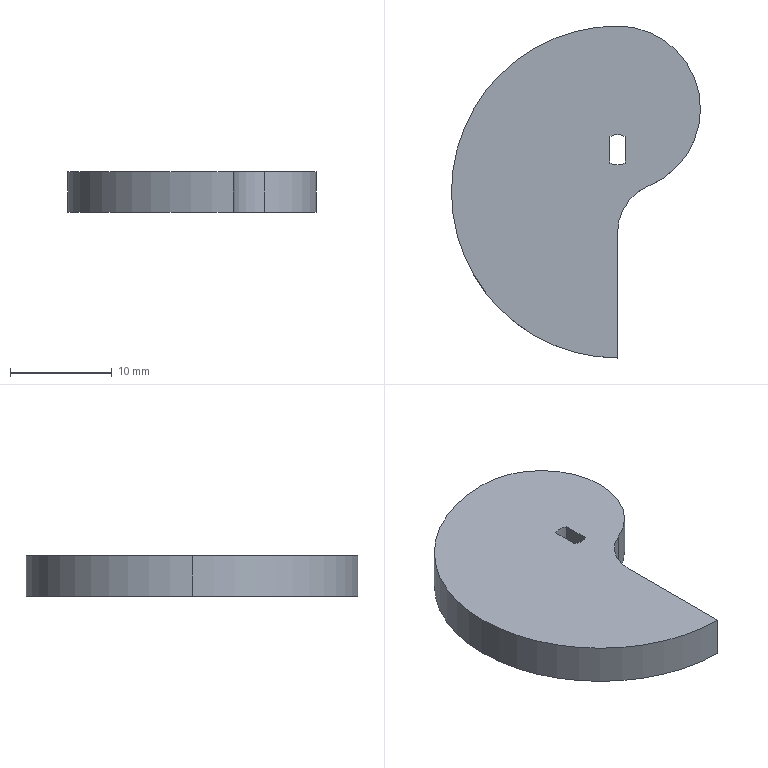Part | SolidWorks | features ICE 4, Attribute 1, Extrusion 1, Fillet 1 | 1 solid | 11 faces | box 24.525 x 32.7 x 4 mm | volume 2093 mm3 | cylinder 6 | plane 5 | commonest cylinder face diameters 3 x2 32.7 x2 10 x1 16.35 x1
STEP:
#1=CARTESIAN_POINT('',(-0.6437,-0.1634,0.1575));
#2=VERTEX_POINT('',#1);
#3=CARTESIAN_POINT('',(0.,-0.8071,0.1575));
#4=VERTEX_POINT('',#3);
#5=CARTESIAN_POINT('',(0.,-0.1634,0.1575));
#6=DIRECTION('',(0.,0.,1.));
#7=DIRECTION('',(1.,0.,0.));
#8=AXIS2_PLACEMENT_3D('',#5,#6,#7);
#9=CIRCLE('',#8,0.6437);
#10=EDGE_CURVE('',#2,#4,#9,.T.);
#11=ORIENTED_EDGE('',*,*,#10,.F.);
#12=CARTESIAN_POINT('',(-0.6437,-0.1634,0.));
#13=VERTEX_POINT('',#12);
#14=CARTESIAN_POINT('',(-0.6437,-0.1634,0.1575));
#15=DIRECTION('',(0.,0.,-1.));
#16=VECTOR('',#15,39.37);
#17=LINE('',#14,#16);
#18=EDGE_CURVE('',#2,#13,#17,.T.);
#19=ORIENTED_EDGE('',*,*,#18,.T.);
#20=CARTESIAN_POINT('',(0.,-0.8071,0.));
#21=VERTEX_POINT('',#20);
#22=CARTESIAN_POINT('',(0.,-0.1634,0.));
#23=DIRECTION('',(0.,0.,1.));
#24=DIRECTION('',(1.,0.,0.));
#25=AXIS2_PLACEMENT_3D('',#22,#23,#24);
#26=CIRCLE('',#25,0.6437);
#27=EDGE_CURVE('',#13,#21,#26,.T.);
#28=ORIENTED_EDGE('',*,*,#27,.T.);
#29=CARTESIAN_POINT('',(0.,-0.8071,0.1575));
#30=DIRECTION('',(0.,0.,-1.));
#31=VECTOR('',#30,39.37);
#32=LINE('',#29,#31);
#33=EDGE_CURVE('',#4,#21,#32,.T.);
#34=ORIENTED_EDGE('',*,*,#33,.F.);
#35=EDGE_LOOP('',(#11,#19,#28,#34));
#36=FACE_OUTER_BOUND('',#35,.T.);
#37=CARTESIAN_POINT('',(0.,-0.1634,0.1575));
#38=DIRECTION('',(0.,0.,-1.));
#39=DIRECTION('',(-1.,0.,0.));
#40=AXIS2_PLACEMENT_3D('',#37,#38,#39);
#41=CYLINDRICAL_SURFACE('',#40,0.6437);
#42=ADVANCED_FACE('',(#36),#41,.T.);
#43=CARTESIAN_POINT('',(-0.02953,-0.05114,0.));
#44=VERTEX_POINT('',#43);
#45=CARTESIAN_POINT('',(-0.02953,-0.05114,0.1575));
#46=VERTEX_POINT('',#45);
#47=CARTESIAN_POINT('',(-0.02953,-0.05114,0.));
#48=DIRECTION('',(0.,0.,1.));
#49=VECTOR('',#48,39.37);
#50=LINE('',#47,#49);
#51=EDGE_CURVE('',#44,#46,#50,.T.);
#52=ORIENTED_EDGE('',*,*,#51,.T.);
#53=CARTESIAN_POINT('',(0.02953,-0.05114,0.1575));
#54=VERTEX_POINT('',#53);
#55=CARTESIAN_POINT('',(0.,0.,0.1575));
#56=DIRECTION('',(0.,0.,1.));
#57=DIRECTION('',(1.,0.,0.));
#58=AXIS2_PLACEMENT_3D('',#55,#56,#57);
#59=CIRCLE('',#58,0.05906);
#60=EDGE_CURVE('',#46,#54,#59,.T.);
#61=ORIENTED_EDGE('',*,*,#60,.T.);
#62=CARTESIAN_POINT('',(0.02953,-0.05114,0.));
#63=VERTEX_POINT('',#62);
#64=CARTESIAN_POINT('',(0.02953,-0.05114,0.));
#65=DIRECTION('',(0.,0.,1.));
#66=VECTOR('',#65,39.37);
#67=LINE('',#64,#66);
#68=EDGE_CURVE('',#63,#54,#67,.T.);
#69=ORIENTED_EDGE('',*,*,#68,.F.);
#70=CARTESIAN_POINT('',(0.,0.,0.));
#71=DIRECTION('',(0.,0.,1.));
#72=DIRECTION('',(1.,0.,0.));
#73=AXIS2_PLACEMENT_3D('',#70,#71,#72);
#74=CIRCLE('',#73,0.05906);
#75=EDGE_CURVE('',#44,#63,#74,.T.);
#76=ORIENTED_EDGE('',*,*,#75,.F.);
#77=EDGE_LOOP('',(#52,#61,#69,#76));
#78=FACE_OUTER_BOUND('',#77,.T.);
#79=CARTESIAN_POINT('',(0.,0.,0.));
#80=DIRECTION('',(0.,0.,1.));
#81=DIRECTION('',(1.,0.,0.));
#82=AXIS2_PLACEMENT_3D('',#79,#80,#81);
#83=CYLINDRICAL_SURFACE('',#82,0.05906);
#84=ADVANCED_FACE('',(#78),#83,.F.);
#85=CARTESIAN_POINT('',(-0.02953,0.05114,0.));
#86=VERTEX_POINT('',#85);
#87=CARTESIAN_POINT('',(-0.02953,0.05114,0.1575));
#88=VERTEX_POINT('',#87);
#89=CARTESIAN_POINT('',(-0.02953,0.05114,0.));
#90=DIRECTION('',(0.,0.,1.));
#91=VECTOR('',#90,39.37);
#92=LINE('',#89,#91);
#93=EDGE_CURVE('',#86,#88,#92,.T.);
#94=ORIENTED_EDGE('',*,*,#93,.F.);
#95=CARTESIAN_POINT('',(0.02953,0.05114,0.));
#96=VERTEX_POINT('',#95);
#97=CARTESIAN_POINT('',(0.,0.,0.));
#98=DIRECTION('',(0.,0.,1.));
#99=DIRECTION('',(1.,0.,0.));
#100=AXIS2_PLACEMENT_3D('',#97,#98,#99);
#101=CIRCLE('',#100,0.05906);
#102=EDGE_CURVE('',#96,#86,#101,.T.);
#103=ORIENTED_EDGE('',*,*,#102,.F.);
#104=CARTESIAN_POINT('',(0.02953,0.05114,0.1575));
#105=VERTEX_POINT('',#104);
#106=CARTESIAN_POINT('',(0.02953,0.05114,0.));
#107=DIRECTION('',(0.,0.,1.));
#108=VECTOR('',#107,39.37);
#109=LINE('',#106,#108);
#110=EDGE_CURVE('',#96,#105,#109,.T.);
#111=ORIENTED_EDGE('',*,*,#110,.T.);
#112=CARTESIAN_POINT('',(0.,0.,0.1575));
#113=DIRECTION('',(0.,0.,1.));
#114=DIRECTION('',(1.,0.,0.));
#115=AXIS2_PLACEMENT_3D('',#112,#113,#114);
#116=CIRCLE('',#115,0.05906);
#117=EDGE_CURVE('',#105,#88,#116,.T.);
#118=ORIENTED_EDGE('',*,*,#117,.T.);
#119=EDGE_LOOP('',(#94,#103,#111,#118));
#120=FACE_OUTER_BOUND('',#119,.T.);
#121=CARTESIAN_POINT('',(0.,0.,0.));
#122=DIRECTION('',(0.,0.,1.));
#123=DIRECTION('',(1.,0.,0.));
#124=AXIS2_PLACEMENT_3D('',#121,#122,#123);
#125=CYLINDRICAL_SURFACE('',#124,0.05906);
#126=ADVANCED_FACE('',(#120),#125,.F.);
#127=CARTESIAN_POINT('',(0.,-0.3214,0.));
#128=VERTEX_POINT('',#127);
#129=CARTESIAN_POINT('',(0.,-0.3214,0.1575));
#130=VERTEX_POINT('',#129);
#131=CARTESIAN_POINT('',(0.,-0.3214,0.1575));
#132=DIRECTION('',(0.,0.,1.));
#133=VECTOR('',#132,39.37);
#134=LINE('',#131,#133);
#135=EDGE_CURVE('',#128,#130,#134,.T.);
#136=ORIENTED_EDGE('',*,*,#135,.F.);
#137=CARTESIAN_POINT('',(0.1221,-0.1393,0.));
#138=VERTEX_POINT('',#137);
#139=CARTESIAN_POINT('',(0.1969,-0.3214,0.));
#140=DIRECTION('',(0.,0.,-1.));
#141=DIRECTION('',(1.,0.,0.));
#142=AXIS2_PLACEMENT_3D('',#139,#140,#141);
#143=CIRCLE('',#142,0.1969);
#144=EDGE_CURVE('',#128,#138,#143,.T.);
#145=ORIENTED_EDGE('',*,*,#144,.T.);
#146=CARTESIAN_POINT('',(0.1221,-0.1393,0.1575));
#147=VERTEX_POINT('',#146);
#148=CARTESIAN_POINT('',(0.1221,-0.1393,0.1575));
#149=DIRECTION('',(0.,0.,-1.));
#150=VECTOR('',#149,39.37);
#151=LINE('',#148,#150);
#152=EDGE_CURVE('',#147,#138,#151,.T.);
#153=ORIENTED_EDGE('',*,*,#152,.F.);
#154=CARTESIAN_POINT('',(0.1969,-0.3214,0.1575));
#155=DIRECTION('',(0.,0.,1.));
#156=DIRECTION('',(1.,0.,0.));
#157=AXIS2_PLACEMENT_3D('',#154,#155,#156);
#158=CIRCLE('',#157,0.1969);
#159=EDGE_CURVE('',#147,#130,#158,.T.);
#160=ORIENTED_EDGE('',*,*,#159,.T.);
#161=EDGE_LOOP('',(#136,#145,#153,#160));
#162=FACE_OUTER_BOUND('',#161,.T.);
#163=CARTESIAN_POINT('',(0.1969,-0.3214,0.1575));
#164=DIRECTION('',(0.,0.,-1.));
#165=DIRECTION('',(-1.,0.,0.));
#166=AXIS2_PLACEMENT_3D('',#163,#164,#165);
#167=CYLINDRICAL_SURFACE('',#166,0.1969);
#168=ADVANCED_FACE('',(#162),#167,.F.);
#169=ORIENTED_EDGE('',*,*,#117,.F.);
#170=CARTESIAN_POINT('',(0.02953,0.,0.1575));
#171=DIRECTION('',(0.,-1.,0.));
#172=VECTOR('',#171,39.37);
#173=LINE('',#170,#172);
#174=EDGE_CURVE('',#105,#54,#173,.T.);
#175=ORIENTED_EDGE('',*,*,#174,.T.);
#176=ORIENTED_EDGE('',*,*,#60,.F.);
#177=CARTESIAN_POINT('',(-0.02953,0.,0.1575));
#178=DIRECTION('',(0.,-1.,0.));
#179=VECTOR('',#178,39.37);
#180=LINE('',#177,#179);
#181=EDGE_CURVE('',#88,#46,#180,.T.);
#182=ORIENTED_EDGE('',*,*,#181,.F.);
#183=EDGE_LOOP('',(#169,#175,#176,#182));
#184=FACE_BOUND('',#183,.T.);
#185=ORIENTED_EDGE('',*,*,#159,.F.);
#186=CARTESIAN_POINT('',(0.,0.4803,0.1575));
#187=VERTEX_POINT('',#186);
#188=CARTESIAN_POINT('',(0.,0.1585,0.1575));
#189=DIRECTION('',(0.,0.,1.));
#190=DIRECTION('',(1.,0.,0.));
#191=AXIS2_PLACEMENT_3D('',#188,#189,#190);
#192=CIRCLE('',#191,0.3219);
#193=EDGE_CURVE('',#147,#187,#192,.T.);
#194=ORIENTED_EDGE('',*,*,#193,.T.);
#195=CARTESIAN_POINT('',(0.,-0.1634,0.1575));
#196=DIRECTION('',(0.,0.,1.));
#197=DIRECTION('',(1.,0.,0.));
#198=AXIS2_PLACEMENT_3D('',#195,#196,#197);
#199=CIRCLE('',#198,0.6437);
#200=EDGE_CURVE('',#187,#2,#199,.T.);
#201=ORIENTED_EDGE('',*,*,#200,.T.);
#202=ORIENTED_EDGE('',*,*,#10,.T.);
#203=CARTESIAN_POINT('',(0.,-0.8071,0.1575));
#204=DIRECTION('',(0.,1.,0.));
#205=VECTOR('',#204,39.37);
#206=LINE('',#203,#205);
#207=EDGE_CURVE('',#4,#130,#206,.T.);
#208=ORIENTED_EDGE('',*,*,#207,.T.);
#209=EDGE_LOOP('',(#185,#194,#201,#202,#208));
#210=FACE_OUTER_BOUND('',#209,.T.);
#211=CARTESIAN_POINT('',(0.,0.1585,0.1575));
#212=DIRECTION('',(0.,0.,1.));
#213=DIRECTION('',(1.,0.,0.));
#214=AXIS2_PLACEMENT_3D('',#211,#212,#213);
#215=PLANE('',#214);
#216=ADVANCED_FACE('',(#184,#210),#215,.T.);
#217=ORIENTED_EDGE('',*,*,#102,.T.);
#218=CARTESIAN_POINT('',(-0.02953,0.,0.));
#219=DIRECTION('',(0.,-1.,0.));
#220=VECTOR('',#219,39.37);
#221=LINE('',#218,#220);
#222=EDGE_CURVE('',#86,#44,#221,.T.);
#223=ORIENTED_EDGE('',*,*,#222,.T.);
#224=ORIENTED_EDGE('',*,*,#75,.T.);
#225=CARTESIAN_POINT('',(0.02953,0.,0.));
#226=DIRECTION('',(0.,-1.,0.));
#227=VECTOR('',#226,39.37);
#228=LINE('',#225,#227);
#229=EDGE_CURVE('',#96,#63,#228,.T.);
#230=ORIENTED_EDGE('',*,*,#229,.F.);
#231=EDGE_LOOP('',(#217,#223,#224,#230));
#232=FACE_BOUND('',#231,.T.);
#233=CARTESIAN_POINT('',(0.,0.4803,0.));
#234=VERTEX_POINT('',#233);
#235=CARTESIAN_POINT('',(0.,0.1585,0.));
#236=DIRECTION('',(0.,0.,1.));
#237=DIRECTION('',(1.,0.,0.));
#238=AXIS2_PLACEMENT_3D('',#235,#236,#237);
#239=CIRCLE('',#238,0.3219);
#240=EDGE_CURVE('',#138,#234,#239,.T.);
#241=ORIENTED_EDGE('',*,*,#240,.F.);
#242=ORIENTED_EDGE('',*,*,#144,.F.);
#243=CARTESIAN_POINT('',(0.,-0.8071,0.));
#244=DIRECTION('',(0.,1.,0.));
#245=VECTOR('',#244,39.37);
#246=LINE('',#243,#245);
#247=EDGE_CURVE('',#21,#128,#246,.T.);
#248=ORIENTED_EDGE('',*,*,#247,.F.);
#249=ORIENTED_EDGE('',*,*,#27,.F.);
#250=CARTESIAN_POINT('',(0.,-0.1634,0.));
#251=DIRECTION('',(0.,0.,1.));
#252=DIRECTION('',(1.,0.,0.));
#253=AXIS2_PLACEMENT_3D('',#250,#251,#252);
#254=CIRCLE('',#253,0.6437);
#255=EDGE_CURVE('',#234,#13,#254,.T.);
#256=ORIENTED_EDGE('',*,*,#255,.F.);
#257=EDGE_LOOP('',(#241,#242,#248,#249,#256));
#258=FACE_OUTER_BOUND('',#257,.T.);
#259=CARTESIAN_POINT('',(0.,0.1585,0.));
#260=DIRECTION('',(0.,0.,1.));
#261=DIRECTION('',(1.,0.,0.));
#262=AXIS2_PLACEMENT_3D('',#259,#260,#261);
#263=PLANE('',#262);
#264=ADVANCED_FACE('',(#232,#258),#263,.F.);
#265=ORIENTED_EDGE('',*,*,#193,.F.);
#266=ORIENTED_EDGE('',*,*,#152,.T.);
#267=ORIENTED_EDGE('',*,*,#240,.T.);
#268=CARTESIAN_POINT('',(0.,0.4803,0.1575));
#269=DIRECTION('',(0.,0.,-1.));
#270=VECTOR('',#269,39.37);
#271=LINE('',#268,#270);
#272=EDGE_CURVE('',#187,#234,#271,.T.);
#273=ORIENTED_EDGE('',*,*,#272,.F.);
#274=EDGE_LOOP('',(#265,#266,#267,#273));
#275=FACE_OUTER_BOUND('',#274,.T.);
#276=CARTESIAN_POINT('',(0.,0.1585,0.1575));
#277=DIRECTION('',(0.,0.,-1.));
#278=DIRECTION('',(-1.,0.,0.));
#279=AXIS2_PLACEMENT_3D('',#276,#277,#278);
#280=CYLINDRICAL_SURFACE('',#279,0.3219);
#281=ADVANCED_FACE('',(#275),#280,.T.);
#282=ORIENTED_EDGE('',*,*,#18,.F.);
#283=ORIENTED_EDGE('',*,*,#200,.F.);
#284=ORIENTED_EDGE('',*,*,#272,.T.);
#285=ORIENTED_EDGE('',*,*,#255,.T.);
#286=EDGE_LOOP('',(#282,#283,#284,#285));
#287=FACE_OUTER_BOUND('',#286,.T.);
#288=CARTESIAN_POINT('',(0.,-0.1634,0.1575));
#289=DIRECTION('',(0.,0.,-1.));
#290=DIRECTION('',(-1.,0.,0.));
#291=AXIS2_PLACEMENT_3D('',#288,#289,#290);
#292=CYLINDRICAL_SURFACE('',#291,0.6437);
#293=ADVANCED_FACE('',(#287),#292,.T.);
#294=ORIENTED_EDGE('',*,*,#247,.T.);
#295=ORIENTED_EDGE('',*,*,#135,.T.);
#296=ORIENTED_EDGE('',*,*,#207,.F.);
#297=ORIENTED_EDGE('',*,*,#33,.T.);
#298=EDGE_LOOP('',(#294,#295,#296,#297));
#299=FACE_OUTER_BOUND('',#298,.T.);
#300=CARTESIAN_POINT('',(0.,-0.8071,0.1575));
#301=DIRECTION('',(-1.,0.,0.));
#302=DIRECTION('',(0.,0.,1.));
#303=AXIS2_PLACEMENT_3D('',#300,#301,#302);
#304=PLANE('',#303);
#305=ADVANCED_FACE('',(#299),#304,.F.);
#306=ORIENTED_EDGE('',*,*,#174,.F.);
#307=ORIENTED_EDGE('',*,*,#110,.F.);
#308=ORIENTED_EDGE('',*,*,#229,.T.);
#309=ORIENTED_EDGE('',*,*,#68,.T.);
#310=EDGE_LOOP('',(#306,#307,#308,#309));
#311=FACE_OUTER_BOUND('',#310,.T.);
#312=CARTESIAN_POINT('',(0.02953,0.,0.));
#313=DIRECTION('',(-1.,0.,0.));
#314=DIRECTION('',(0.,0.,1.));
#315=AXIS2_PLACEMENT_3D('',#312,#313,#314);
#316=PLANE('',#315);
#317=ADVANCED_FACE('',(#311),#316,.T.);
#318=ORIENTED_EDGE('',*,*,#181,.T.);
#319=ORIENTED_EDGE('',*,*,#51,.F.);
#320=ORIENTED_EDGE('',*,*,#222,.F.);
#321=ORIENTED_EDGE('',*,*,#93,.T.);
#322=EDGE_LOOP('',(#318,#319,#320,#321));
#323=FACE_OUTER_BOUND('',#322,.T.);
#324=CARTESIAN_POINT('',(-0.02953,0.,0.));
#325=DIRECTION('',(-1.,0.,0.));
#326=DIRECTION('',(0.,0.,1.));
#327=AXIS2_PLACEMENT_3D('',#324,#325,#326);
#328=PLANE('',#327);
#329=ADVANCED_FACE('',(#323),#328,.F.);
#330=CLOSED_SHELL('',(#42,#84,#126,#168,#216,#264,#281,#293,#305,#317,#329));
#331=MANIFOLD_SOLID_BREP('',#330);
#332=CARTESIAN_POINT('',(0.,0.,0.));
#333=DIRECTION('',(0.,0.,1.));
#334=DIRECTION('',(1.,0.,0.));
#335=AXIS2_PLACEMENT_3D('',#332,#333,#334);
#336=(LENGTH_UNIT()NAMED_UNIT(*)SI_UNIT($,.METRE.));
#337=LENGTH_MEASURE_WITH_UNIT(LENGTH_MEASURE(0.0254),#336);
#338=DIMENSIONAL_EXPONENTS(1.,0.,0.,0.,0.,0.,0.);
#339=(CONVERSION_BASED_UNIT('INCH',#337)LENGTH_UNIT()NAMED_UNIT(#338));
#340=UNCERTAINTY_MEASURE_WITH_UNIT(LENGTH_MEASURE(0.00001),#339,'','');
#341=(NAMED_UNIT(*)PLANE_ANGLE_UNIT()SI_UNIT($,.RADIAN.));
#342=(NAMED_UNIT(*)SI_UNIT($,.STERADIAN.)SOLID_ANGLE_UNIT());
#343=(GEOMETRIC_REPRESENTATION_CONTEXT(3)GLOBAL_UNCERTAINTY_ASSIGNED_CONTEXT((#340))GLOBAL_UNIT_ASSIGNED_CONTEXT((#339,#341,#342))REPRESENTATION_CONTEXT('',''));
#344=ADVANCED_BREP_SHAPE_REPRESENTATION('',(#331,#335),#343);